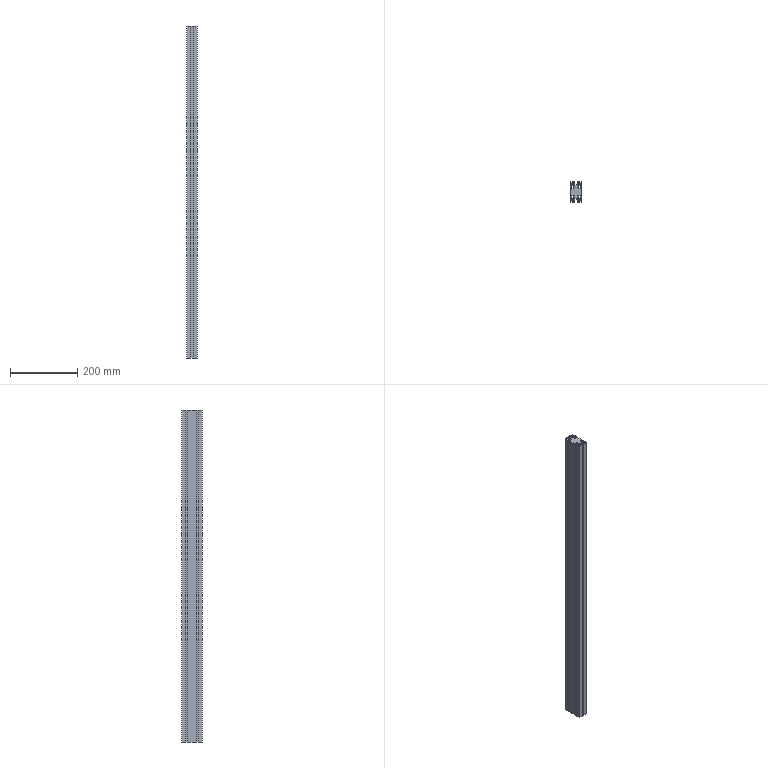Part | SolidWorks | features Extrusion 1 | 1 solid | 86 faces | box 30 x 60 x 990 mm | volume 1191103 mm3 | plane 78 | cylinder 8 | commonest cylinder face diameters 6 x8